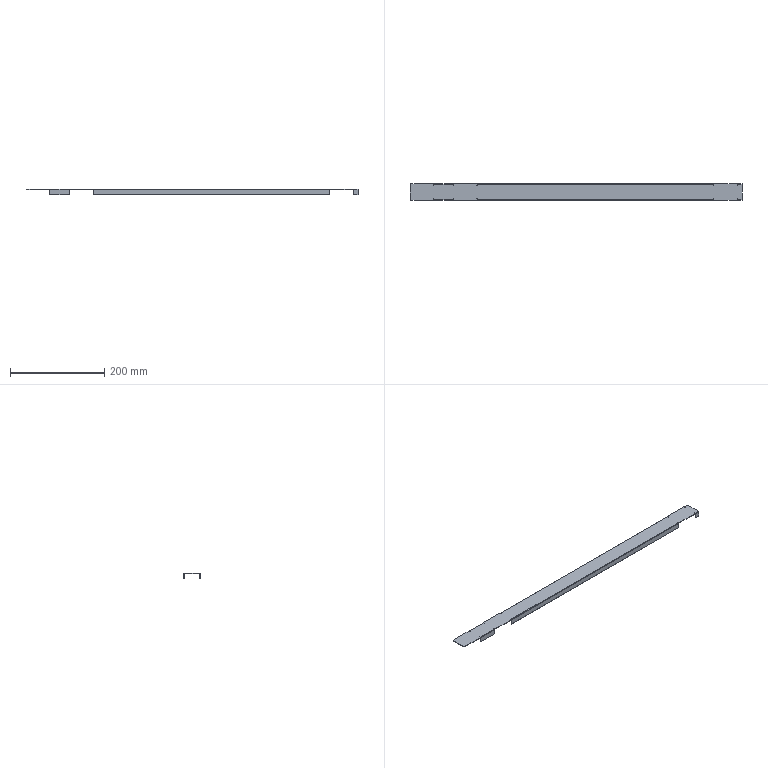Part | SolidWorks | features SMBaseFlange 2, Chamfer 1, Cut 1, EdgeFlange 1, FlatPattern 1, ICE 1, MirrorPattern 1, SheetMetal 1 | 1 solid | 96 faces | box 703.5 x 34 x 12 mm | volume 35744 mm3 | plane 84 | cylinder 12 | commonest cylinder face diameters 0.4 x6 2.4 x6